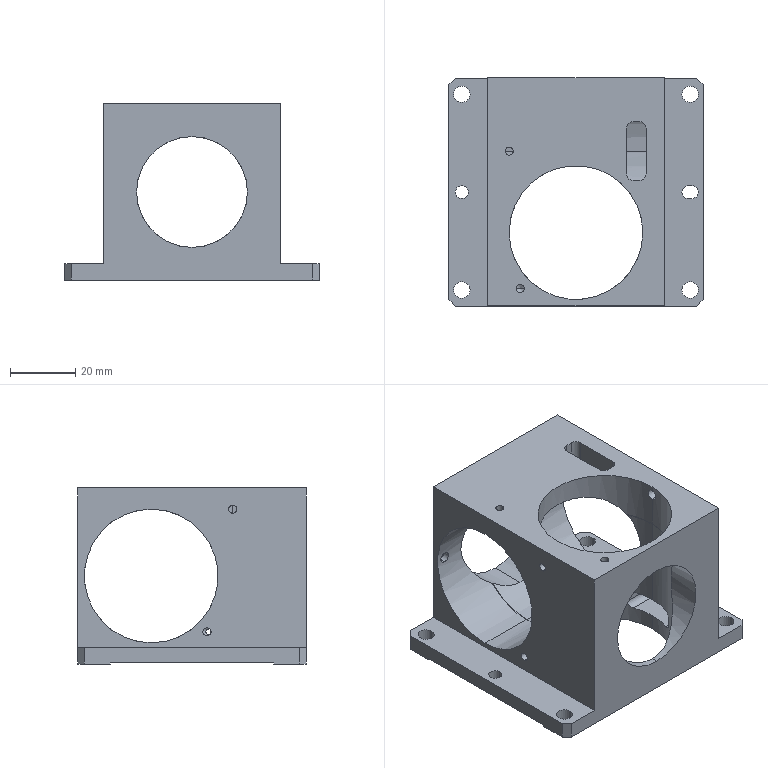NC program | NX | posted with a generic post | part box 78 x 70 x 54 mm
Lines 4370 to 5040 of 5040:
(FLOOR_WALL_1_COPY , TOOL : D16JING)
N8714 T13 M6
N8716 G54
N8718 G17 G0 G90 X-40.771 Y-44.947 B0. C0. S9500 M3
N8720 G43 Z30. H13
N8722 Z-49.
N8724 G94 G1 X-39.799 Y-44.386 F1000.
N8726 G3 X-38.999 Y-43. R1.6
N8728 G1 Y43. F1200.
N8730 X-35.95
N8732 Y-43.
N8734 G2 X-36.75 Y-44.386 R1.6
N8736 G1 X-37.814 Y-45.
N8738 X-37.15 Y-45.078
N8740 X-35.95 Y-44.386 F1000.
N8742 G3 X-35.15 Y-43. R1.6
N8744 G1 Y43. F1200.
N8746 G3 X-35.95 Y44.386 R1.6
N8748 G1 X-37.15 Y45.078
N8750 G0 Z30.
N8752 X40.771 Y44.947
N8754 Z-49.
N8756 G1 X39.799 Y44.386 F1000.
N8758 G3 X38.999 Y43. R1.6
N8760 G1 Y-43. F1200.
N8762 X35.95
N8764 Y43.
N8766 G2 X36.75 Y44.386 R1.6
N8768 G1 X37.814 Y45.
N8770 X37.15 Y45.078
N8772 X35.95 Y44.386 F1000.
N8774 G3 X35.15 Y43. R1.6
N8776 G1 Y-43. F1200.
N8778 G3 X35.95 Y-44.386 R1.6
N8780 G1 X37.15 Y-45.078
N8782 G0 Z30.
(FLOOR_WALL_1_COPY_COPY , TOOL : D16JING)
N8784 X-37. Y-37.078
N8786 Z-4.
N8788 G1 X-35.8 Y-36.386 F1000.
N8790 G3 X-35. Y-35. R1.6
N8792 G1 Y35. F1200.
N8794 G3 X-35.8 Y36.386 R1.6
N8796 G1 X-37. Y37.078
N8798 G0 Y-37.078 Z-13.
N8800 G1 X-35.8 Y-36.386 F1000.
N8802 G3 X-35. Y-35. R1.6
N8804 G1 Y35. F1200.
N8806 G3 X-35.8 Y36.386 R1.6
N8808 G1 X-37. Y37.078
N8810 G0 Y-37.078 Z-22.
N8812 G1 X-35.8 Y-36.386 F1000.
N8814 G3 X-35. Y-35. R1.6
N8816 G1 Y35. F1200.
N8818 G3 X-35.8 Y36.386 R1.6
N8820 G1 X-37. Y37.078
N8822 G0 Y-37.078 Z-31.
N8824 G1 X-35.8 Y-36.386 F1000.
N8826 G3 X-35. Y-35. R1.6
N8828 G1 Y35. F1200.
N8830 G3 X-35.8 Y36.386 R1.6
N8832 G1 X-37. Y37.078
N8834 G0 Y-37.078 Z-40.
N8836 G1 X-35.8 Y-36.386 F1000.
N8838 G3 X-35. Y-35. R1.6
N8840 G1 Y35. F1200.
N8842 G3 X-35.8 Y36.386 R1.6
N8844 G1 X-37. Y37.078
N8846 G0 Y-37.078 Z-49.
N8848 G1 X-35.8 Y-36.386 F1000.
N8850 G3 X-35. Y-35. R1.6
N8852 G1 Y35. F1200.
N8854 G3 X-35.8 Y36.386 R1.6
N8856 G1 X-37. Y37.078
N8858 G0 Z30.
N8860 X37.
N8862 Z-4.
N8864 G1 X35.8 Y36.386 F1000.
N8866 G3 X35. Y35. R1.6
N8868 G1 Y-35. F1200.
N8870 G3 X35.8 Y-36.386 R1.6
N8872 G1 X37. Y-37.078
N8874 G0 Y37.078 Z-13.
N8876 G1 X35.8 Y36.386 F1000.
N8878 G3 X35. Y35. R1.6
N8880 G1 Y-35. F1200.
N8882 G3 X35.8 Y-36.386 R1.6
N8884 G1 X37. Y-37.078
N8886 G0 Y37.078 Z-22.
N8888 G1 X35.8 Y36.386 F1000.
N8890 G3 X35. Y35. R1.6
N8892 G1 Y-35. F1200.
N8894 G3 X35.8 Y-36.386 R1.6
N8896 G1 X37. Y-37.078
N8898 G0 Y37.078 Z-31.
N8900 G1 X35.8 Y36.386 F1000.
N8902 G3 X35. Y35. R1.6
N8904 G1 Y-35. F1200.
N8906 G3 X35.8 Y-36.386 R1.6
N8908 G1 X37. Y-37.078
N8910 G0 Y37.078 Z-40.
N8912 G1 X35.8 Y36.386 F1000.
N8914 G3 X35. Y35. R1.6
N8916 G1 Y-35. F1200.
N8918 G3 X35.8 Y-36.386 R1.6
N8920 G1 X37. Y-37.078
N8922 G0 Y37.078 Z-49.
N8924 G1 X35.8 Y36.386 F1000.
N8926 G3 X35. Y35. R1.6
N8928 G1 Y-35. F1200.
N8930 G3 X35.8 Y-36.386 R1.6
N8932 G1 X37. Y-37.078
N8934 G0 Z30.
(CAVITY_MILL_COPY_1 , TOOL : D16JING)
N8936 X-37.964 Y-37.288
N8938 Z-12.5
N8940 G1 Z-13.5 F1000.
N8942 X-35.5 Y-35.866
N8944 G3 X-35. Y-35. R1.
N8946 G1 Y35. F1200.
N8948 G2 X-27. Y43. R8.
N8950 G1 X27.
N8952 G2 X35. Y35. R8.
N8954 G1 Y-35.
N8956 G2 X27. Y-43. R8.
N8958 G1 X-27.
N8960 G2 X-35. Y-35. R8.
N8962 G3 X-35.5 Y-34.134 R1.
N8964 G1 X-38.2 Y-32.575
N8966 Z-12.5
N8968 G0 Z30.
N8970 X39.288 Y-45.964
N8972 Z-26.
N8974 G1 Z-27. F1000.
N8976 X37.866 Y-43.5
N8978 G3 X37. Y-43. R1.
N8980 G1 X-37. F1200.
N8982 G2 X-42.657 Y-40.657 R8.
N8984 G1 X-44.657 Y-38.657
N8986 G2 X-47. Y-33. R8.
N8988 G1 Y33.
N8990 G2 X-44.657 Y38.657 R8.
N8992 G1 X-42.657 Y40.657
N8994 G2 X-37. Y43. R8.
N8996 G1 X37.
N8998 G2 X42.657 Y40.657 R8.
N9000 G1 X44.657 Y38.657
N9002 G2 X47. Y33. R8.
N9004 G1 Y-33.
N9006 G2 X44.657 Y-38.657 R8.
N9008 G1 X42.657 Y-40.657
N9010 G2 X37. Y-43. R8.
N9012 G3 X36.134 Y-43.5 R1.
N9014 G1 X34.575 Y-46.2
N9016 Z-26.
N9018 G0 Z-10.5
N9020 X39.288 Y-45.964
N9022 Z-39.5
N9024 G1 Z-40.5 F1000.
N9026 X37.866 Y-43.5
N9028 G3 X37. Y-43. R1.
N9030 G1 X-37. F1200.
N9032 G2 X-42.657 Y-40.657 R8.
N9034 G1 X-44.657 Y-38.657
N9036 G2 X-47. Y-33. R8.
N9038 G1 Y33.
N9040 G2 X-44.657 Y38.657 R8.
N9042 G1 X-42.657 Y40.657
N9044 G2 X-37. Y43. R8.
N9046 G1 X37.
N9048 G2 X42.657 Y40.657 R8.
N9050 G1 X44.657 Y38.657
N9052 G2 X47. Y33. R8.
N9054 G1 Y-33.
N9056 G2 X44.657 Y-38.657 R8.
N9058 G1 X42.657 Y-40.657
N9060 G2 X37. Y-43. R8.
N9062 G3 X36.134 Y-43.5 R1.
N9064 G1 X34.575 Y-46.2
N9066 Z-39.5
N9068 G0 Z-24.
N9070 X39.288 Y-45.964
N9072 Z-53.
N9074 G1 Z-54. F1000.
N9076 X37.866 Y-43.5
N9078 G3 X37. Y-43. R1.
N9080 G1 X-37. F1200.
N9082 G2 X-42.657 Y-40.657 R8.
N9084 G1 X-44.657 Y-38.657
N9086 G2 X-47. Y-33. R8.
N9088 G1 Y33.
N9090 G2 X-44.657 Y38.657 R8.
N9092 G1 X-42.657 Y40.657
N9094 G2 X-37. Y43. R8.
N9096 G1 X37.
N9098 G2 X42.657 Y40.657 R8.
N9100 G1 X44.657 Y38.657
N9102 G2 X47. Y33. R8.
N9104 G1 Y-33.
N9106 G2 X44.657 Y-38.657 R8.
N9108 G1 X42.657 Y-40.657
N9110 G2 X37. Y-43. R8.
N9112 G3 X36.134 Y-43.5 R1.
N9114 G1 X34.575 Y-46.2
N9116 Z-53.
N9118 G0 Z30.
N9120 M5
(ZLEVEL_PROFILE_1 , TOOL : D4)
N9122 T04 M6
N9124 G54
N9126 G17 G0 G90 X19.5 Y18.92 B0. C0. S9500 M3
N9128 G43 Z30. H4
N9130 Z1.
N9132 G94 G1 Y19.493 Z0.97 F1250.
N9134 X19.471 Y19.5 Z0.968
N9136 X17.529 Z0.867
N9138 X17.5 Y19.493 Z0.865
N9140 Y5.547 Z0.134
N9142 X17.51 Y5.5 Z0.132
N9144 X19.492 Z0.028
N9146 X19.5 Y5.547 Z0.025
N9148 Y12.496 Z-0.339
N9150 Y19.493
N9152 X19.471 Y19.5
N9154 X17.529
N9156 X17.5 Y19.493
N9158 Y5.547
N9160 X17.51 Y5.5
N9162 X19.492
N9164 X19.5 Y5.547
N9166 Y12.496
N9168 Y19.251 Z-0.457
N9170 X19.499 Y19.416 Z-0.46
N9172 X19.491 Y19.491 Z-0.461
N9174 X19.461 Y19.5 Z-0.462
N9176 X17.773 Z-0.491
N9178 X17.515 Y19.492 Z-0.496
N9180 X17.507 Y19.485
N9182 X17.5 Y19.345 Z-0.499
N9184 Y9.071 Z-0.678
N9186 Y5.547
N9188 X17.51 Y5.5
N9190 X19.492
N9192 X19.5 Y5.547
N9194 Y12.496
N9196 Y19.251 Z-0.796
N9198 X19.499 Y19.416 Z-0.799
N9200 X19.491 Y19.491 Z-0.8
N9202 X19.487 Y19.5
N9204 X19.321 Z-0.803
N9206 X17.773 Z-0.83
N9208 X17.515 Y19.492 Z-0.835
N9210 X17.507 Y19.485
N9212 X17.5 Y19.345 Z-0.838
N9214 Y9.071 Z-1.017
N9216 Y5.547
N9218 X17.51 Y5.5
N9220 X19.492
N9222 X19.5 Y5.547
N9224 Y12.496
N9226 Y19.251 Z-1.135
N9228 X19.499 Y19.416 Z-1.138
N9230 X19.491 Y19.491 Z-1.139
N9232 X19.487 Y19.5
N9234 X19.321 Z-1.142
N9236 X17.773 Z-1.169
N9238 X17.515 Y19.492 Z-1.174
N9240 X17.507 Y19.485
N9242 X17.5 Y19.345 Z-1.177
N9244 Y9.071 Z-1.356
N9246 Y5.547
N9248 X17.51 Y5.5
N9250 X19.492
N9252 X19.5 Y5.547
N9254 Y12.496
N9256 Y19.251 Z-1.474
N9258 X19.499 Y19.416 Z-1.477
N9260 X19.491 Y19.491 Z-1.478
N9262 X19.487 Y19.5
N9264 X19.321 Z-1.481
N9266 X17.773 Z-1.508
N9268 X17.596 Z-1.511
N9270 X17.511 Y19.492 Z-1.513
N9272 X17.507 Y19.485
N9274 X17.5 Y19.345 Z-1.516
N9276 Y9.071 Z-1.695
N9278 Y5.547
N9280 X17.51 Y5.5
N9282 X19.492
N9284 X19.5 Y5.547
N9286 Y12.496
N9288 Y19.251 Z-1.813
N9290 X19.499 Y19.416 Z-1.816
N9292 X19.491 Y19.491 Z-1.817
N9294 X19.487 Y19.5
N9296 X19.321 Z-1.82
N9298 X17.773 Z-1.847
N9300 X17.596 Z-1.85
N9302 X17.511 Y19.492 Z-1.852
N9304 X17.507 Y19.485
N9306 X17.5 Y19.345 Z-1.855
N9308 Y9.071 Z-2.034
N9310 Y5.547
N9312 X17.51 Y5.5
N9314 X19.492
N9316 X19.5 Y5.547
N9318 Y12.496
N9320 Y19.251 Z-2.152
N9322 X19.499 Y19.416 Z-2.155
N9324 X19.491 Y19.491 Z-2.156
N9326 X19.487 Y19.5
N9328 X19.321 Z-2.159
N9330 X17.773 Z-2.186
N9332 X17.596 Z-2.189
N9334 X17.511 Y19.492 Z-2.191
N9336 X17.507 Y19.485
N9338 X17.5 Y19.344 Z-2.194
N9340 Y9.071 Z-2.373
N9342 Y5.547
N9344 X17.51 Y5.5
N9346 X19.492
N9348 X19.5 Y5.547
N9350 Y12.496
N9352 Y19.251 Z-2.491
N9354 X19.499 Y19.416 Z-2.494
N9356 X19.491 Y19.491 Z-2.495
N9358 X19.487 Y19.5
N9360 X19.32 Z-2.498
N9362 X19.18 Z-2.501
N9364 X17.772 Z-2.525
N9366 X17.596 Z-2.528
N9368 X17.516 Z-2.53
N9370 X17.507 Y19.485
N9372 X17.5 Y19.344 Z-2.533
N9374 Y9.071 Z-2.712
N9376 Y5.547
N9378 X17.51 Y5.5
N9380 X19.492
N9382 X19.5 Y5.547
N9384 Y12.496
N9386 Y19.251 Z-2.83
N9388 X19.499 Y19.416 Z-2.833
N9390 X19.491 Y19.491 Z-2.834
N9392 X19.487 Y19.5
N9394 X19.32 Z-2.837
N9396 X19.18 Z-2.84
N9398 X17.772 Z-2.864
N9400 X17.596 Z-2.867
N9402 X17.516 Z-2.869
N9404 X17.507 Y19.485
N9406 X17.5 Y19.344 Z-2.872
N9408 Y9.071 Z-3.051
N9410 Y5.547
N9412 X17.51 Y5.5
N9414 X19.492
N9416 X19.5 Y5.547
N9418 Y12.496
N9420 Y19.251 Z-3.169
N9422 X19.499 Y19.416 Z-3.172
N9424 X19.491 Y19.491 Z-3.173
N9426 X19.487 Y19.5
N9428 X19.32 Z-3.176
N9430 X19.18 Z-3.179
N9432 X17.772 Z-3.203
N9434 X17.596 Z-3.206
N9436 X17.516 Z-3.208
N9438 X17.507 Y19.485
N9440 X17.5 Y19.344 Z-3.211
N9442 Y9.071 Z-3.39
N9444 Y5.547
N9446 X17.51 Y5.5
N9448 X19.492
N9450 X19.5 Y5.547
N9452 Y12.496
N9454 Y19.251 Z-3.508
N9456 X19.499 Y19.416 Z-3.511
N9458 X19.491 Y19.491 Z-3.512
N9460 X19.487 Y19.5
N9462 X19.32 Z-3.515
N9464 X19.18 Z-3.518
N9466 X17.772 Z-3.542
N9468 X17.596 Z-3.545
N9470 X17.516 Z-3.547
N9472 X17.507 Y19.485
N9474 X17.5 Y19.344 Z-3.55
N9476 Y9.071 Z-3.729
N9478 Y5.547
N9480 X17.51 Y5.5
N9482 X19.492
N9484 X19.5 Y5.547
N9486 Y12.496
N9488 Y19.251 Z-3.847
N9490 X19.499 Y19.416 Z-3.85
N9492 X19.491 Y19.491 Z-3.851
N9494 X19.487 Y19.5
N9496 X19.32 Z-3.854
N9498 X19.18 Z-3.857
N9500 X17.772 Z-3.881
N9502 X17.596 Z-3.884
N9504 X17.516 Z-3.886
N9506 X17.507 Y19.485
N9508 X17.5 Y19.344 Z-3.889
N9510 Y9.071 Z-4.068
N9512 Y5.547
N9514 X17.51 Y5.5
N9516 X19.492
N9518 X19.5 Y5.547
N9520 Y12.496
N9522 Y19.251 Z-4.186
N9524 X19.499 Y19.416 Z-4.189
N9526 X19.491 Y19.491 Z-4.19
N9528 X19.461 Y19.5 Z-4.191
N9530 X19.18 Z-4.196
N9532 X17.772 Z-4.22
N9534 X17.596 Z-4.223
N9536 X17.516 Z-4.225
N9538 X17.507 Y19.485
N9540 X17.5 Y19.344 Z-4.227
N9542 Y9.071 Z-4.407
N9544 Y5.547
N9546 X17.51 Y5.5
N9548 X19.492
N9550 X19.5 Y5.547
N9552 Y12.496
N9554 Y19.251 Z-4.525
N9556 X19.499 Y19.416 Z-4.528
N9558 X19.491 Y19.491 Z-4.529
N9560 X19.461 Y19.5 Z-4.53
N9562 X19.18 Z-4.535
N9564 X17.772 Z-4.559
N9566 X17.596 Z-4.562
N9568 X17.516 Z-4.564
N9570 X17.507 Y19.485
N9572 X17.5 Y19.344 Z-4.566
N9574 Y9.071 Z-4.746
N9576 Y5.547
N9578 X17.51 Y5.5
N9580 X19.492
N9582 X19.5 Y5.547
N9584 Y12.496
N9586 Y19.251 Z-4.864
N9588 X19.499 Y19.416 Z-4.867
N9590 X19.491 Y19.491 Z-4.868
N9592 X19.461 Y19.5 Z-4.869
N9594 X19.18 Z-4.874
N9596 X17.772 Z-4.898
N9598 X17.596 Z-4.901
N9600 X17.516 Z-4.903
N9602 X17.507 Y19.485
N9604 X17.5 Y19.344 Z-4.905
N9606 Y9.071 Z-5.085
N9608 Y5.547
N9610 X17.51 Y5.5
N9612 X19.492
N9614 X19.5 Y5.547
N9616 Y12.496
N9618 Y19.251 Z-5.203
N9620 X19.499 Y19.416 Z-5.206
N9622 X19.491 Y19.491 Z-5.207
N9624 X19.461 Y19.5 Z-5.208
N9626 X19.18 Z-5.213
N9628 X17.772 Z-5.237
N9630 X17.596 Z-5.24
N9632 X17.516 Z-5.242
N9634 X17.507 Y19.485
N9636 X17.5 Y19.344 Z-5.244
N9638 Y9.071 Z-5.424
N9640 Y5.547
N9642 X17.51 Y5.5
N9644 X19.492
N9646 X19.5 Y5.547
N9648 Y12.496
N9650 Y19.251 Z-5.542
N9652 X19.499 Y19.416 Z-5.545
N9654 X19.491 Y19.491 Z-5.546
N9656 X19.461 Y19.5 Z-5.547
N9658 X19.18 Z-5.552
N9660 X17.772 Z-5.576
N9662 X17.596 Z-5.579
N9664 X17.516 Z-5.581
N9666 X17.507 Y19.485
N9668 X17.5 Y19.344 Z-5.583
N9670 Y9.071 Z-5.763
N9672 Y5.547
N9674 X17.51 Y5.5
N9676 X19.492
N9678 X19.5 Y5.547
N9680 Y12.496
N9682 Y19.251 Z-5.881
N9684 X19.499 Y19.416 Z-5.883
N9686 X19.491 Y19.491 Z-5.885
N9688 X19.461 Y19.5 Z-5.886
N9690 X19.18 Z-5.89
N9692 X17.772 Z-5.915
N9694 X17.596 Z-5.918
N9696 X17.516 Z-5.92
N9698 X17.507 Y19.485
N9700 X17.5 Y19.344 Z-5.922
N9702 Y9.071 Z-6.102
N9704 Y5.547
N9706 X17.51 Y5.5
N9708 X19.492
N9710 X19.5 Y5.547
N9712 Y12.496
N9714 Y19.251 Z-6.22
N9716 X19.499 Y19.416 Z-6.222
N9718 X19.491 Y19.491 Z-6.224
N9720 X19.461 Y19.5 Z-6.225
N9722 X19.18 Z-6.229
N9724 X17.772 Z-6.254
N9726 X17.596 Z-6.257
N9728 X17.516 Z-6.259
N9730 X17.507 Y19.485
N9732 X17.5 Y19.344 Z-6.261
N9734 Y9.071 Z-6.441
N9736 Y5.547
N9738 X17.51 Y5.5
N9740 X19.492
N9742 X19.5 Y5.547
N9744 Y12.496
N9746 Y19.251 Z-6.559
N9748 X19.499 Y19.416 Z-6.561
N9750 X19.491 Y19.491 Z-6.563
N9752 X19.461 Y19.5 Z-6.564
N9754 X19.18 Z-6.568
N9756 X17.772 Z-6.593
N9758 X17.596 Z-6.596
N9760 X17.516 Z-6.598
N9762 X17.507 Y19.485
N9764 X17.5 Y19.344 Z-6.6
N9766 Y9.071 Z-6.78
N9768 Y5.547
N9770 X17.51 Y5.5
N9772 X19.492
N9774 X19.5 Y5.547
N9776 Y12.496
N9778 Y19.251 Z-6.898
N9780 X19.499 Y19.416 Z-6.9
N9782 X19.491 Y19.491 Z-6.902
N9784 X19.461 Y19.5 Z-6.903
N9786 X19.179 Z-6.907
N9788 X17.772 Z-6.932
N9790 X17.596 Z-6.935
N9792 X17.516 Z-6.937
N9794 X17.507 Y19.485
N9796 X17.5 Y19.344 Z-6.939
N9798 Y9.071 Z-7.119
N9800 Y5.547
N9802 X17.51 Y5.5
N9804 X19.492
N9806 X19.5 Y5.547
N9808 Y12.496
N9810 Y19.251 Z-7.237
N9812 X19.499 Y19.416 Z-7.239
N9814 X19.491 Y19.491 Z-7.241
N9816 X19.461 Y19.5 Z-7.242
N9818 X19.179 Z-7.246
N9820 X17.772 Z-7.271
N9822 X17.596 Z-7.274
N9824 X17.51 Y19.492 Z-7.276
N9826 X17.507 Y19.484
N9828 X17.5 Y19.344 Z-7.278
N9830 Y9.071 Z-7.458
N9832 Y5.547
N9834 X17.51 Y5.5
N9836 X19.492
N9838 X19.5 Y5.547
N9840 Y12.496
N9842 Y19.251 Z-7.576
N9844 X19.499 Y19.416 Z-7.578
N9846 X19.491 Y19.491 Z-7.58
N9848 X19.461 Y19.5 Z-7.581
N9850 X19.179 Z-7.585
N9852 X17.772 Z-7.61
N9854 X17.596 Z-7.613
N9856 X17.51 Y19.492 Z-7.615
N9858 X17.507 Y19.484
N9860 X17.5 Y19.344 Z-7.617
N9862 Y9.071 Z-7.797
N9864 Y5.547
N9866 X17.51 Y5.5
N9868 X19.492
N9870 X19.5 Y5.547
N9872 Y12.496
N9874 Y19.251 Z-7.915
N9876 X19.499 Y19.416 Z-7.917
N9878 X19.491 Y19.491 Z-7.919
N9880 X19.461 Y19.5
N9882 X19.179 Z-7.924
N9884 X17.772 Z-7.949
N9886 X17.596 Z-7.952
N9888 X17.51 Y19.492 Z-7.954
N9890 X17.507 Y19.484
N9892 X17.5 Y19.344 Z-7.956
N9894 Y9.071 Z-8.136
N9896 Y5.547
N9898 X17.51 Y5.5
N9900 X19.492
N9902 X19.5 Y5.547
N9904 Y12.496
N9906 Y19.251 Z-8.254
N9908 X19.499 Y19.416 Z-8.256
N9910 X19.491 Y19.491 Z-8.258
N9912 X19.461 Y19.5
N9914 X19.179 Z-8.263
N9916 X17.772 Z-8.288
N9918 X17.596 Z-8.291
N9920 X17.51 Y19.492 Z-8.293
N9922 X17.507 Y19.484
N9924 X17.5 Y19.344 Z-8.295
N9926 Y9.071 Z-8.475
N9928 Y5.547
N9930 X17.51 Y5.5
N9932 X19.492
N9934 X19.5 Y5.547
N9936 Y12.496
N9938 Y19.251 Z-8.593
N9940 X19.499 Y19.416 Z-8.595
N9942 X19.491 Y19.491 Z-8.597
N9944 X19.461 Y19.5
N9946 X19.179 Z-8.602
N9948 X17.772 Z-8.627
N9950 X17.596 Z-8.63
N9952 X17.51 Y19.492 Z-8.632
N9954 X17.507 Y19.484
N9956 X17.5 Y19.344 Z-8.634
N9958 Y9.071 Z-8.814
N9960 Y5.547
N9962 X17.51 Y5.5
N9964 X19.492
N9966 X19.5 Y5.547
N9968 Y19.493
N9970 X19.453 Y19.5
N9972 X17.547
N9974 X17.5 Y19.486
N9976 Y9.071
N9978 Z-7.814
N9980 G0 Z30.
N9982 M5
(TOOLCOMP , TOOL : D16JING)
N9984 T13 M6
N9986 G54
N9988 G17 G0 G90 X0. Y-12.5 B0. C0. S9500 M3
N9990 G43 Z30. H13
N9992 Z0.5
N9994 G41 G94 G1 X8.894 Y-15.543 F1000. D13
N9996 G3 X12.45 Y-12.5 R3.08
N9998 X12.45 Y-12.5 Z-9.5 I-12.45 J0.
N10000 X12.45 Y-12.5 Z-19.5 I-12.45 J0.
N10002 X12.45 Y-12.5 Z-29.5 I-12.45 J0.
N10004 X12.45 Y-12.5 Z-39.5 I-12.45 J0.
N10006 X12.45 Y-12.5 Z-49.5 I-12.45 J0.
N10008 X-11.841 Y-8.653 Z-54. R12.45
N10010 X-3.847 Y-24.341 R12.45
N10012 X-11.841 Y-8.653 R-12.45
N10014 X-9.399 Y-12.646 R3.08
N10016 G40
N10018 G1 X0. Y-12.5
N10020 G0 Z30.
N10022 M5
N10024 M2